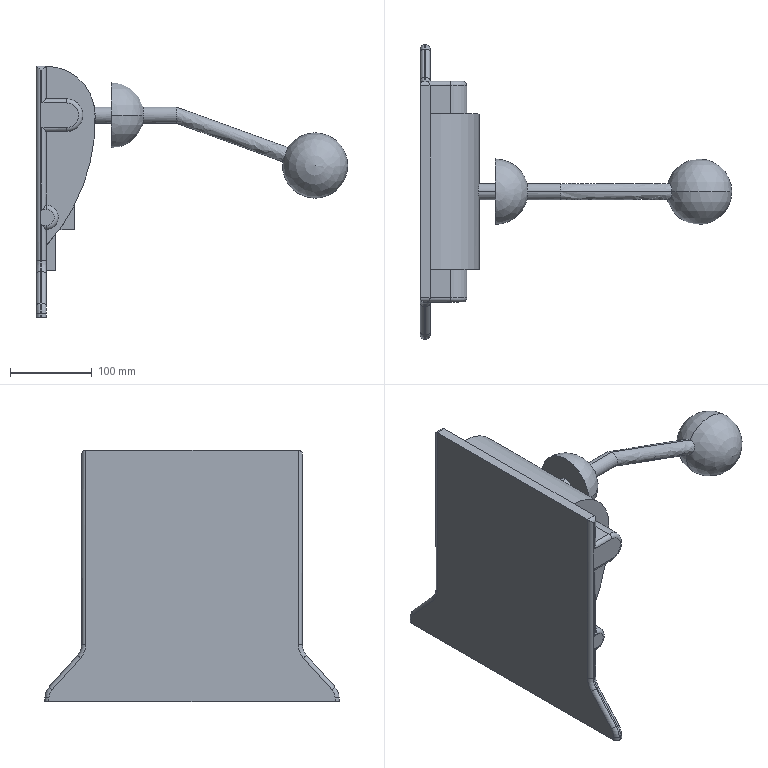Part | SolidWorks | 1 solid | 88 faces | box 381.145 x 360 x 307.969 mm | volume 3545128 mm3 | cylinder 36 | plane 30 | torus 16 | sphere 4 | spline 2 | commonest cylinder face diameters 10 x22 40 x6 20 x4 30 x2 120 x1 460 x1